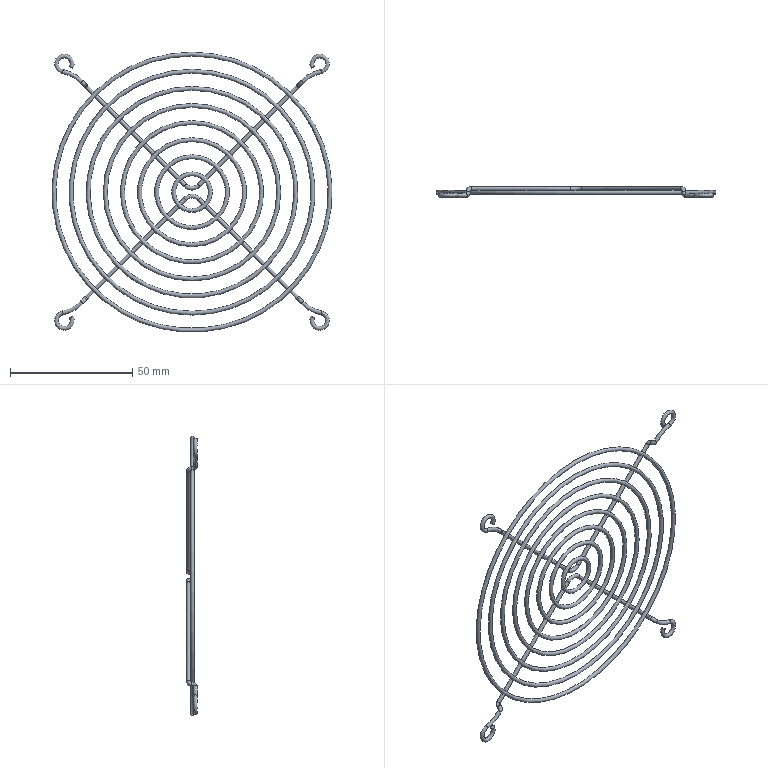Part | NX | features BREP 10 | 10 solids | 42 faces | box 114.6 x 4.4 x 114.6 mm | volume 3954 mm3 | torus 26 | plane 12 | cylinder 4 | commonest cylinder face diameters 1.6 x4
STEP:
#1=CARTESIAN_POINT('',(-52.712,-1.2,-50.143));
#2=VERTEX_POINT('',#1);
#3=CARTESIAN_POINT('',(-52.862,-1.2,-49.357));
#4=DIRECTION('',(-0.9823,0.,-0.1875));
#5=DIRECTION('',(0.1875,0.,-0.9823));
#6=AXIS2_PLACEMENT_3D('',#3,#4,#5);
#7=CIRCLE('',#6,0.8);
#8=EDGE_CURVE('',#2,#2,#7,.T.);
#9=ORIENTED_EDGE('',*,*,#8,.F.);
#10=EDGE_LOOP('',(#9));
#11=FACE_BOUND('',#10,.T.);
#12=CARTESIAN_POINT('',(-45.113,-0.4,-45.113));
#13=VERTEX_POINT('',#12);
#14=CARTESIAN_POINT('',(-44.532,-1.2,-45.663));
#15=VERTEX_POINT('',#14);
#16=CARTESIAN_POINT('',(-45.113,-0.4,-45.113));
#17=CARTESIAN_POINT('',(-44.809,-0.4,-45.401));
#18=CARTESIAN_POINT('',(-44.532,-0.7811,-45.663));
#19=CARTESIAN_POINT('',(-44.532,-1.2,-45.663));
#20=B_SPLINE_CURVE_WITH_KNOTS('',3,(#16,#17,#18,#19),.UNSPECIFIED.,.F.,.F.,(4,4),(0.,1.),.UNSPECIFIED.);
#21=EDGE_CURVE('',#13,#15,#20,.T.);
#22=ORIENTED_EDGE('',*,*,#21,.T.);
#23=CARTESIAN_POINT('',(-45.113,-2.,-45.113));
#24=VERTEX_POINT('',#23);
#25=CARTESIAN_POINT('',(-44.54,-1.2,-45.671));
#26=CARTESIAN_POINT('',(-44.539,-1.623,-45.671));
#27=CARTESIAN_POINT('',(-44.812,-2.,-45.405));
#28=CARTESIAN_POINT('',(-45.113,-2.,-45.113));
#29=B_SPLINE_CURVE_WITH_KNOTS('',3,(#25,#26,#27,#28),.UNSPECIFIED.,.F.,.F.,(4,4),(0.,0.001252),.UNSPECIFIED.);
#30=EDGE_CURVE('',#15,#24,#29,.T.);
#31=ORIENTED_EDGE('',*,*,#30,.T.);
#32=CARTESIAN_POINT('',(-45.113,-1.2,-45.113));
#33=DIRECTION('',(-0.687,0.,-0.7266));
#34=DIRECTION('',(0.7266,0.,-0.687));
#35=AXIS2_PLACEMENT_3D('',#32,#33,#34);
#36=CIRCLE('',#35,0.8);
#37=EDGE_CURVE('',#24,#13,#36,.T.);
#38=ORIENTED_EDGE('',*,*,#37,.T.);
#39=EDGE_LOOP('',(#22,#31,#38));
#40=FACE_BOUND('',#39,.T.);
#41=CARTESIAN_POINT('',(-55.558,-1.2,-35.238));
#42=DIRECTION('',(0.,1.,0.));
#43=DIRECTION('',(0.,0.,-1.));
#44=AXIS2_PLACEMENT_3D('',#41,#42,#43);
#45=TOROIDAL_SURFACE('',#44,14.374,0.8);
#46=ADVANCED_FACE('',(#11,#40),#45,.T.);
#47=CARTESIAN_POINT('',(-50.126,-1.2,-51.405));
#48=VERTEX_POINT('',#47);
#49=CARTESIAN_POINT('',(-49.414,-1.2,-51.04));
#50=DIRECTION('',(-0.4563,0.,0.8898));
#51=DIRECTION('',(-0.8898,0.,-0.4563));
#52=AXIS2_PLACEMENT_3D('',#49,#50,#51);
#53=CIRCLE('',#52,0.8);
#54=EDGE_CURVE('',#48,#48,#53,.T.);
#55=ORIENTED_EDGE('',*,*,#54,.F.);
#56=EDGE_LOOP('',(#55));
#57=FACE_BOUND('',#56,.T.);
#58=ORIENTED_EDGE('',*,*,#8,.T.);
#59=EDGE_LOOP('',(#58));
#60=FACE_BOUND('',#59,.T.);
#61=CARTESIAN_POINT('',(-52.262,-1.2,-52.5));
#62=DIRECTION('',(0.,-1.,0.));
#63=DIRECTION('',(0.,0.,1.));
#64=AXIS2_PLACEMENT_3D('',#61,#62,#63);
#65=TOROIDAL_SURFACE('',#64,3.2,0.8);
#66=ADVANCED_FACE('',(#57,#60),#65,.T.);
#67=CARTESIAN_POINT('',(-43.558,0.2,-44.689));
#68=VERTEX_POINT('',#67);
#69=CARTESIAN_POINT('',(-44.123,0.2,-44.123));
#70=DIRECTION('',(0.,-1.,0.));
#71=DIRECTION('',(0.7071,0.,-0.7071));
#72=AXIS2_PLACEMENT_3D('',#69,#70,#71);
#73=CIRCLE('',#72,0.8);
#74=EDGE_CURVE('',#68,#68,#73,.T.);
#75=ORIENTED_EDGE('',*,*,#74,.T.);
#76=EDGE_LOOP('',(#75));
#77=FACE_BOUND('',#76,.T.);
#78=CARTESIAN_POINT('',(-45.113,-1.2,-45.113));
#79=DIRECTION('',(-0.7071,0.,-0.7071));
#80=DIRECTION('',(0.7071,0.,-0.7071));
#81=AXIS2_PLACEMENT_3D('',#78,#79,#80);
#82=CIRCLE('',#81,0.8);
#83=EDGE_CURVE('',#24,#13,#82,.T.);
#84=ORIENTED_EDGE('',*,*,#83,.F.);
#85=ORIENTED_EDGE('',*,*,#30,.F.);
#86=ORIENTED_EDGE('',*,*,#21,.F.);
#87=EDGE_LOOP('',(#84,#85,#86));
#88=FACE_BOUND('',#87,.T.);
#89=CARTESIAN_POINT('',(-45.113,0.2,-45.113));
#90=DIRECTION('',(-0.7071,0.,0.7071));
#91=DIRECTION('',(-0.7071,0.,-0.7071));
#92=AXIS2_PLACEMENT_3D('',#89,#90,#91);
#93=TOROIDAL_SURFACE('',#92,1.4,0.8);
#94=ADVANCED_FACE('',(#77,#88),#93,.T.);
#95=CARTESIAN_POINT('',(-42.568,1.6,-43.699));
#96=VERTEX_POINT('',#95);
#97=CARTESIAN_POINT('',(-43.134,1.6,-43.134));
#98=DIRECTION('',(0.7071,0.,0.7071));
#99=DIRECTION('',(0.7071,0.,-0.7071));
#100=AXIS2_PLACEMENT_3D('',#97,#98,#99);
#101=CIRCLE('',#100,0.8);
#102=EDGE_CURVE('',#96,#96,#101,.T.);
#103=ORIENTED_EDGE('',*,*,#102,.F.);
#104=EDGE_LOOP('',(#103));
#105=FACE_BOUND('',#104,.T.);
#106=ORIENTED_EDGE('',*,*,#74,.F.);
#107=EDGE_LOOP('',(#106));
#108=FACE_BOUND('',#107,.T.);
#109=CARTESIAN_POINT('',(-43.134,0.2,-43.134));
#110=DIRECTION('',(0.7071,0.,-0.7071));
#111=DIRECTION('',(0.7071,0.,0.7071));
#112=AXIS2_PLACEMENT_3D('',#109,#110,#111);
#113=TOROIDAL_SURFACE('',#112,1.4,0.8);
#114=ADVANCED_FACE('',(#105,#108),#113,.T.);
#115=CARTESIAN_POINT('',(50.126,-1.2,-51.405));
#116=VERTEX_POINT('',#115);
#117=CARTESIAN_POINT('',(49.414,-1.2,-51.04));
#118=DIRECTION('',(0.4563,0.,0.8898));
#119=DIRECTION('',(0.8898,0.,-0.4563));
#120=AXIS2_PLACEMENT_3D('',#117,#118,#119);
#121=CIRCLE('',#120,0.8);
#122=EDGE_CURVE('',#116,#116,#121,.T.);
#123=ORIENTED_EDGE('',*,*,#122,.F.);
#124=EDGE_LOOP('',(#123));
#125=FACE_BOUND('',#124,.T.);
#126=CARTESIAN_POINT('',(52.712,-1.2,-50.143));
#127=VERTEX_POINT('',#126);
#128=CARTESIAN_POINT('',(52.862,-1.2,-49.357));
#129=DIRECTION('',(0.9823,0.,-0.1875));
#130=DIRECTION('',(-0.1875,0.,-0.9823));
#131=AXIS2_PLACEMENT_3D('',#128,#129,#130);
#132=CIRCLE('',#131,0.8);
#133=EDGE_CURVE('',#127,#127,#132,.T.);
#134=ORIENTED_EDGE('',*,*,#133,.T.);
#135=EDGE_LOOP('',(#134));
#136=FACE_BOUND('',#135,.T.);
#137=CARTESIAN_POINT('',(52.262,-1.2,-52.5));
#138=DIRECTION('',(0.,1.,0.));
#139=DIRECTION('',(0.,0.,-1.));
#140=AXIS2_PLACEMENT_3D('',#137,#138,#139);
#141=TOROIDAL_SURFACE('',#140,3.2,0.8);
#142=ADVANCED_FACE('',(#125,#136),#141,.T.);
#143=ORIENTED_EDGE('',*,*,#133,.F.);
#144=EDGE_LOOP('',(#143));
#145=FACE_BOUND('',#144,.T.);
#146=CARTESIAN_POINT('',(45.113,-2.,-45.113));
#147=VERTEX_POINT('',#146);
#148=CARTESIAN_POINT('',(44.538,-1.2,-45.67));
#149=VERTEX_POINT('',#148);
#150=CARTESIAN_POINT('',(45.113,-2.,-45.113));
#151=CARTESIAN_POINT('',(44.906,-2.,-45.321));
#152=CARTESIAN_POINT('',(44.583,-1.678,-45.641));
#153=CARTESIAN_POINT('',(44.542,-1.326,-45.674));
#154=CARTESIAN_POINT('',(44.539,-1.2,-45.67));
#155=B_SPLINE_CURVE_WITH_KNOTS('',3,(#150,#151,#152,#153,#154),.UNSPECIFIED.,.F.,.F.,(4,1,4),(0.,0.5,1.),.UNSPECIFIED.);
#156=EDGE_CURVE('',#147,#149,#155,.T.);
#157=ORIENTED_EDGE('',*,*,#156,.T.);
#158=CARTESIAN_POINT('',(45.113,-0.4,-45.113));
#159=VERTEX_POINT('',#158);
#160=CARTESIAN_POINT('',(44.54,-1.2,-45.671));
#161=CARTESIAN_POINT('',(44.54,-0.7768,-45.672));
#162=CARTESIAN_POINT('',(44.814,-0.4,-45.407));
#163=CARTESIAN_POINT('',(45.113,-0.4,-45.113));
#164=B_SPLINE_CURVE_WITH_KNOTS('',3,(#160,#161,#162,#163),.UNSPECIFIED.,.F.,.F.,(4,4),(0.000000002,0.001252),.UNSPECIFIED.);
#165=EDGE_CURVE('',#149,#159,#164,.T.);
#166=ORIENTED_EDGE('',*,*,#165,.T.);
#167=CARTESIAN_POINT('',(45.113,-1.2,-45.113));
#168=DIRECTION('',(0.687,0.,-0.7266));
#169=DIRECTION('',(0.7266,0.,0.687));
#170=AXIS2_PLACEMENT_3D('',#167,#168,#169);
#171=CIRCLE('',#170,0.8);
#172=EDGE_CURVE('',#159,#147,#171,.T.);
#173=ORIENTED_EDGE('',*,*,#172,.T.);
#174=EDGE_LOOP('',(#157,#166,#173));
#175=FACE_BOUND('',#174,.T.);
#176=CARTESIAN_POINT('',(55.558,-1.2,-35.238));
#177=DIRECTION('',(0.,-1.,0.));
#178=DIRECTION('',(0.,0.,1.));
#179=AXIS2_PLACEMENT_3D('',#176,#177,#178);
#180=TOROIDAL_SURFACE('',#179,14.374,0.8);
#181=ADVANCED_FACE('',(#145,#175),#180,.T.);
#182=CARTESIAN_POINT('',(43.558,0.2,-44.689));
#183=VERTEX_POINT('',#182);
#184=CARTESIAN_POINT('',(44.123,0.2,-44.123));
#185=DIRECTION('',(0.,-1.,0.));
#186=DIRECTION('',(-0.7071,0.,-0.7071));
#187=AXIS2_PLACEMENT_3D('',#184,#185,#186);
#188=CIRCLE('',#187,0.8);
#189=EDGE_CURVE('',#183,#183,#188,.T.);
#190=ORIENTED_EDGE('',*,*,#189,.T.);
#191=EDGE_LOOP('',(#190));
#192=FACE_BOUND('',#191,.T.);
#193=ORIENTED_EDGE('',*,*,#156,.F.);
#194=CARTESIAN_POINT('',(45.113,-1.2,-45.113));
#195=DIRECTION('',(0.7071,0.,-0.7071));
#196=DIRECTION('',(-0.7071,0.,-0.7071));
#197=AXIS2_PLACEMENT_3D('',#194,#195,#196);
#198=CIRCLE('',#197,0.8);
#199=EDGE_CURVE('',#159,#147,#198,.T.);
#200=ORIENTED_EDGE('',*,*,#199,.F.);
#201=ORIENTED_EDGE('',*,*,#165,.F.);
#202=EDGE_LOOP('',(#193,#200,#201));
#203=FACE_BOUND('',#202,.T.);
#204=CARTESIAN_POINT('',(45.113,0.2,-45.113));
#205=DIRECTION('',(-0.7071,0.,-0.7071));
#206=DIRECTION('',(0.7071,0.,-0.7071));
#207=AXIS2_PLACEMENT_3D('',#204,#205,#206);
#208=TOROIDAL_SURFACE('',#207,1.4,0.8);
#209=ADVANCED_FACE('',(#192,#203),#208,.T.);
#210=CARTESIAN_POINT('',(42.568,1.6,-43.699));
#211=VERTEX_POINT('',#210);
#212=CARTESIAN_POINT('',(43.134,1.6,-43.134));
#213=DIRECTION('',(0.7071,0.,-0.7071));
#214=DIRECTION('',(-0.7071,0.,-0.7071));
#215=AXIS2_PLACEMENT_3D('',#212,#213,#214);
#216=CIRCLE('',#215,0.8);
#217=EDGE_CURVE('',#211,#211,#216,.T.);
#218=ORIENTED_EDGE('',*,*,#217,.T.);
#219=EDGE_LOOP('',(#218));
#220=FACE_BOUND('',#219,.T.);
#221=ORIENTED_EDGE('',*,*,#189,.F.);
#222=EDGE_LOOP('',(#221));
#223=FACE_BOUND('',#222,.T.);
#224=CARTESIAN_POINT('',(43.134,0.2,-43.134));
#225=DIRECTION('',(0.7071,0.,0.7071));
#226=DIRECTION('',(-0.7071,0.,0.7071));
#227=AXIS2_PLACEMENT_3D('',#224,#225,#226);
#228=TOROIDAL_SURFACE('',#227,1.4,0.8);
#229=ADVANCED_FACE('',(#220,#223),#228,.T.);
#230=CARTESIAN_POINT('',(2.263,1.6,-3.394));
#231=VERTEX_POINT('',#230);
#232=CARTESIAN_POINT('',(2.828,1.6,-2.828));
#233=DIRECTION('',(0.7071,0.,-0.7071));
#234=DIRECTION('',(-0.7071,0.,-0.7071));
#235=AXIS2_PLACEMENT_3D('',#232,#233,#234);
#236=CIRCLE('',#235,0.8);
#237=EDGE_CURVE('',#231,#231,#236,.T.);
#238=ORIENTED_EDGE('',*,*,#237,.F.);
#239=EDGE_LOOP('',(#238));
#240=FACE_BOUND('',#239,.T.);
#241=CARTESIAN_POINT('',(-2.263,1.6,-3.394));
#242=VERTEX_POINT('',#241);
#243=CARTESIAN_POINT('',(-2.828,1.6,-2.828));
#244=DIRECTION('',(0.7071,0.,0.7071));
#245=DIRECTION('',(0.7071,0.,-0.7071));
#246=AXIS2_PLACEMENT_3D('',#243,#244,#245);
#247=CIRCLE('',#246,0.8);
#248=EDGE_CURVE('',#242,#242,#247,.T.);
#249=ORIENTED_EDGE('',*,*,#248,.T.);
#250=EDGE_LOOP('',(#249));
#251=FACE_BOUND('',#250,.T.);
#252=CARTESIAN_POINT('',(0.,1.6,-5.657));
#253=DIRECTION('',(0.,1.,0.));
#254=DIRECTION('',(0.,0.,-1.));
#255=AXIS2_PLACEMENT_3D('',#252,#253,#254);
#256=TOROIDAL_SURFACE('',#255,4.,0.8);
#257=ADVANCED_FACE('',(#240,#251),#256,.T.);
#258=ORIENTED_EDGE('',*,*,#102,.T.);
#259=EDGE_LOOP('',(#258));
#260=FACE_BOUND('',#259,.T.);
#261=ORIENTED_EDGE('',*,*,#248,.F.);
#262=EDGE_LOOP('',(#261));
#263=FACE_BOUND('',#262,.T.);
#264=CARTESIAN_POINT('',(-2.828,1.6,-2.828));
#265=DIRECTION('',(-0.7071,0.,-0.7071));
#266=DIRECTION('',(0.7071,0.,-0.7071));
#267=AXIS2_PLACEMENT_3D('',#264,#265,#266);
#268=CYLINDRICAL_SURFACE('',#267,0.8);
#269=ADVANCED_FACE('',(#260,#263),#268,.T.);
#270=ORIENTED_EDGE('',*,*,#237,.T.);
#271=EDGE_LOOP('',(#270));
#272=FACE_BOUND('',#271,.T.);
#273=ORIENTED_EDGE('',*,*,#217,.F.);
#274=EDGE_LOOP('',(#273));
#275=FACE_BOUND('',#274,.T.);
#276=CARTESIAN_POINT('',(43.134,1.6,-43.134));
#277=DIRECTION('',(-0.7071,0.,0.7071));
#278=DIRECTION('',(-0.7071,0.,-0.7071));
#279=AXIS2_PLACEMENT_3D('',#276,#277,#278);
#280=CYLINDRICAL_SURFACE('',#279,0.8);
#281=ADVANCED_FACE('',(#272,#275),#280,.T.);
#282=ORIENTED_EDGE('',*,*,#199,.T.);
#283=CARTESIAN_POINT('',(45.113,-1.2,-45.113));
#284=DIRECTION('',(0.,-1.,0.));
#285=VECTOR('',#284,1000.);
#286=LINE('',#283,#285);
#287=EDGE_CURVE('',#159,#147,#286,.T.);
#288=ORIENTED_EDGE('',*,*,#287,.F.);
#289=EDGE_LOOP('',(#282,#288));
#290=FACE_BOUND('',#289,.T.);
#291=CARTESIAN_POINT('',(45.113,-1.2,-45.113));
#292=DIRECTION('',(-0.7071,0.,0.7071));
#293=DIRECTION('',(-0.7071,0.,-0.7071));
#294=AXIS2_PLACEMENT_3D('',#291,#292,#293);
#295=PLANE('',#294);
#296=ADVANCED_FACE('',(#290),#295,.F.);
#297=ORIENTED_EDGE('',*,*,#287,.T.);
#298=ORIENTED_EDGE('',*,*,#172,.F.);
#299=EDGE_LOOP('',(#297,#298));
#300=FACE_BOUND('',#299,.T.);
#301=CARTESIAN_POINT('',(45.113,-1.2,-45.113));
#302=DIRECTION('',(-0.687,0.,0.7266));
#303=DIRECTION('',(-0.7266,0.,-0.687));
#304=AXIS2_PLACEMENT_3D('',#301,#302,#303);
#305=PLANE('',#304);
#306=ADVANCED_FACE('',(#300),#305,.T.);
#307=ORIENTED_EDGE('',*,*,#122,.T.);
#308=EDGE_LOOP('',(#307));
#309=FACE_BOUND('',#308,.T.);
#310=CARTESIAN_POINT('',(49.414,-1.2,-51.04));
#311=DIRECTION('',(-0.4563,0.,-0.8898));
#312=DIRECTION('',(0.8898,0.,-0.4563));
#313=AXIS2_PLACEMENT_3D('',#310,#311,#312);
#314=PLANE('',#313);
#315=ADVANCED_FACE('',(#309),#314,.F.);
#316=ORIENTED_EDGE('',*,*,#83,.T.);
#317=CARTESIAN_POINT('',(-45.113,-1.2,-45.113));
#318=DIRECTION('',(0.,1.,0.));
#319=VECTOR('',#318,1000.);
#320=LINE('',#317,#319);
#321=EDGE_CURVE('',#24,#13,#320,.T.);
#322=ORIENTED_EDGE('',*,*,#321,.F.);
#323=EDGE_LOOP('',(#316,#322));
#324=FACE_BOUND('',#323,.T.);
#325=CARTESIAN_POINT('',(-45.113,-1.2,-45.113));
#326=DIRECTION('',(0.7071,0.,0.7071));
#327=DIRECTION('',(0.7071,0.,-0.7071));
#328=AXIS2_PLACEMENT_3D('',#325,#326,#327);
#329=PLANE('',#328);
#330=ADVANCED_FACE('',(#324),#329,.F.);
#331=ORIENTED_EDGE('',*,*,#321,.T.);
#332=ORIENTED_EDGE('',*,*,#37,.F.);
#333=EDGE_LOOP('',(#331,#332));
#334=FACE_BOUND('',#333,.T.);
#335=CARTESIAN_POINT('',(-45.113,-1.2,-45.113));
#336=DIRECTION('',(0.687,0.,0.7266));
#337=DIRECTION('',(0.7266,0.,-0.687));
#338=AXIS2_PLACEMENT_3D('',#335,#336,#337);
#339=PLANE('',#338);
#340=ADVANCED_FACE('',(#334),#339,.T.);
#341=ORIENTED_EDGE('',*,*,#54,.T.);
#342=EDGE_LOOP('',(#341));
#343=FACE_BOUND('',#342,.T.);
#344=CARTESIAN_POINT('',(-49.414,-1.2,-51.04));
#345=DIRECTION('',(0.4563,0.,-0.8898));
#346=DIRECTION('',(-0.8898,0.,-0.4563));
#347=AXIS2_PLACEMENT_3D('',#344,#345,#346);
#348=PLANE('',#347);
#349=ADVANCED_FACE('',(#343),#348,.F.);
#350=CLOSED_SHELL('',(#46,#66,#94,#114,#142,#181,#209,#229,#257,#269,#281,#296,#306,#315,#330,#340,#349));
#351=MANIFOLD_SOLID_BREP('',#350);
#352=CARTESIAN_POINT('',(0.,0.,20.7));
#353=VERTEX_POINT('',#352);
#354=VERTEX_LOOP('',#353);
#355=FACE_BOUND('',#354,.T.);
#356=CARTESIAN_POINT('',(0.,0.,0.));
#357=DIRECTION('',(0.,1.,0.));
#358=DIRECTION('',(0.,0.,1.));
#359=AXIS2_PLACEMENT_3D('',#356,#357,#358);
#360=TOROIDAL_SURFACE('',#359,21.5,0.8);
#361=ADVANCED_FACE('',(#355),#360,.T.);
#362=CLOSED_SHELL('',(#361));
#363=MANIFOLD_SOLID_BREP('',#362);
#364=CARTESIAN_POINT('',(0.,0.,27.7));
#365=VERTEX_POINT('',#364);
#366=VERTEX_LOOP('',#365);
#367=FACE_BOUND('',#366,.T.);
#368=CARTESIAN_POINT('',(0.,0.,0.));
#369=DIRECTION('',(0.,1.,0.));
#370=DIRECTION('',(0.,0.,1.));
#371=AXIS2_PLACEMENT_3D('',#368,#369,#370);
#372=TOROIDAL_SURFACE('',#371,28.5,0.8);
#373=ADVANCED_FACE('',(#367),#372,.T.);
#374=CLOSED_SHELL('',(#373));
#375=MANIFOLD_SOLID_BREP('',#374);
#376=CARTESIAN_POINT('',(0.,0.,34.7));
#377=VERTEX_POINT('',#376);
#378=VERTEX_LOOP('',#377);
#379=FACE_BOUND('',#378,.T.);
#380=CARTESIAN_POINT('',(0.,0.,0.));
#381=DIRECTION('',(0.,1.,0.));
#382=DIRECTION('',(0.,0.,1.));
#383=AXIS2_PLACEMENT_3D('',#380,#381,#382);
#384=TOROIDAL_SURFACE('',#383,35.5,0.8);
#385=ADVANCED_FACE('',(#379),#384,.T.);
#386=CLOSED_SHELL('',(#385));
#387=MANIFOLD_SOLID_BREP('',#386);
#388=CARTESIAN_POINT('',(-45.113,-2.,45.113));
#389=VERTEX_POINT('',#388);
#390=CARTESIAN_POINT('',(-45.113,-0.4,45.113));
#391=VERTEX_POINT('',#390);
#392=CARTESIAN_POINT('',(-45.113,-1.2,45.113));
#393=DIRECTION('',(0.687,0.,-0.7266));
#394=DIRECTION('',(0.7266,0.,0.687));
#395=AXIS2_PLACEMENT_3D('',#392,#393,#394);
#396=CIRCLE('',#395,0.8);
#397=EDGE_CURVE('',#389,#391,#396,.T.);
#398=ORIENTED_EDGE('',*,*,#397,.F.);
#399=CARTESIAN_POINT('',(-44.532,-1.2,45.663));
#400=VERTEX_POINT('',#399);
#401=CARTESIAN_POINT('',(-44.54,-1.2,45.671));
#402=CARTESIAN_POINT('',(-44.539,-1.623,45.671));
#403=CARTESIAN_POINT('',(-44.812,-2.,45.405));
#404=CARTESIAN_POINT('',(-45.113,-2.,45.113));
#405=B_SPLINE_CURVE_WITH_KNOTS('',3,(#401,#402,#403,#404),.UNSPECIFIED.,.F.,.F.,(4,4),(0.,0.001252),.UNSPECIFIED.);
#406=EDGE_CURVE('',#400,#389,#405,.T.);
#407=ORIENTED_EDGE('',*,*,#406,.F.);
#408=CARTESIAN_POINT('',(-44.54,-1.2,45.671));
#409=CARTESIAN_POINT('',(-44.54,-0.7768,45.672));
#410=CARTESIAN_POINT('',(-44.814,-0.4,45.407));
#411=CARTESIAN_POINT('',(-45.113,-0.4,45.113));
#412=B_SPLINE_CURVE_WITH_KNOTS('',3,(#408,#409,#410,#411),.UNSPECIFIED.,.F.,.F.,(4,4),(0.000000067,0.001252),.UNSPECIFIED.);
#413=EDGE_CURVE('',#391,#400,#412,.F.);
#414=ORIENTED_EDGE('',*,*,#413,.F.);
#415=EDGE_LOOP('',(#398,#407,#414));
#416=FACE_BOUND('',#415,.T.);
#417=CARTESIAN_POINT('',(-52.712,-1.2,50.143));
#418=VERTEX_POINT('',#417);
#419=CARTESIAN_POINT('',(-52.862,-1.2,49.357));
#420=DIRECTION('',(0.9823,0.,-0.1875));
#421=DIRECTION('',(0.1875,0.,0.9823));
#422=AXIS2_PLACEMENT_3D('',#419,#420,#421);
#423=CIRCLE('',#422,0.8);
#424=EDGE_CURVE('',#418,#418,#423,.T.);
#425=ORIENTED_EDGE('',*,*,#424,.T.);
#426=EDGE_LOOP('',(#425));
#427=FACE_BOUND('',#426,.T.);
#428=CARTESIAN_POINT('',(-55.558,-1.2,35.238));
#429=DIRECTION('',(0.,1.,0.));
#430=DIRECTION('',(0.,0.,1.));
#431=AXIS2_PLACEMENT_3D('',#428,#429,#430);
#432=TOROIDAL_SURFACE('',#431,14.374,0.8);
#433=ADVANCED_FACE('',(#416,#427),#432,.T.);
#434=ORIENTED_EDGE('',*,*,#424,.F.);
#435=EDGE_LOOP('',(#434));
#436=FACE_BOUND('',#435,.T.);
#437=CARTESIAN_POINT('',(-50.126,-1.2,51.405));
#438=VERTEX_POINT('',#437);
#439=CARTESIAN_POINT('',(-49.414,-1.2,51.04));
#440=DIRECTION('',(0.4563,0.,0.8898));
#441=DIRECTION('',(-0.8898,0.,0.4563));
#442=AXIS2_PLACEMENT_3D('',#439,#440,#441);
#443=CIRCLE('',#442,0.8);
#444=EDGE_CURVE('',#438,#438,#443,.T.);
#445=ORIENTED_EDGE('',*,*,#444,.T.);
#446=EDGE_LOOP('',(#445));
#447=FACE_BOUND('',#446,.T.);
#448=CARTESIAN_POINT('',(-52.262,-1.2,52.5));
#449=DIRECTION('',(0.,-1.,0.));
#450=DIRECTION('',(0.,0.,-1.));
#451=AXIS2_PLACEMENT_3D('',#448,#449,#450);
#452=TOROIDAL_SURFACE('',#451,3.2,0.8);
#453=ADVANCED_FACE('',(#436,#447),#452,.T.);
#454=CARTESIAN_POINT('',(-45.113,-1.2,45.113));
#455=DIRECTION('',(0.7071,0.,-0.7071));
#456=DIRECTION('',(0.7071,0.,0.7071));
#457=AXIS2_PLACEMENT_3D('',#454,#455,#456);
#458=CIRCLE('',#457,0.8);
#459=EDGE_CURVE('',#389,#391,#458,.T.);
#460=ORIENTED_EDGE('',*,*,#459,.T.);
#461=ORIENTED_EDGE('',*,*,#413,.T.);
#462=ORIENTED_EDGE('',*,*,#406,.T.);
#463=EDGE_LOOP('',(#460,#461,#462));
#464=FACE_BOUND('',#463,.T.);
#465=CARTESIAN_POINT('',(-43.558,0.2,44.689));
#466=VERTEX_POINT('',#465);
#467=CARTESIAN_POINT('',(-44.123,0.2,44.123));
#468=DIRECTION('',(0.,1.,0.));
#469=DIRECTION('',(0.7071,0.,0.7071));
#470=AXIS2_PLACEMENT_3D('',#467,#468,#469);
#471=CIRCLE('',#470,0.8);
#472=EDGE_CURVE('',#466,#466,#471,.T.);
#473=ORIENTED_EDGE('',*,*,#472,.F.);
#474=EDGE_LOOP('',(#473));
#475=FACE_BOUND('',#474,.T.);
#476=CARTESIAN_POINT('',(-45.113,0.2,45.113));
#477=DIRECTION('',(-0.7071,0.,-0.7071));
#478=DIRECTION('',(-0.7071,0.,0.7071));
#479=AXIS2_PLACEMENT_3D('',#476,#477,#478);
#480=TOROIDAL_SURFACE('',#479,1.4,0.8);
#481=ADVANCED_FACE('',(#464,#475),#480,.T.);
#482=ORIENTED_EDGE('',*,*,#472,.T.);
#483=EDGE_LOOP('',(#482));
#484=FACE_BOUND('',#483,.T.);
#485=CARTESIAN_POINT('',(-42.568,1.6,43.699));
#486=VERTEX_POINT('',#485);
#487=CARTESIAN_POINT('',(-43.134,1.6,43.134));
#488=DIRECTION('',(-0.7071,0.,0.7071));
#489=DIRECTION('',(0.7071,0.,0.7071));
#490=AXIS2_PLACEMENT_3D('',#487,#488,#489);
#491=CIRCLE('',#490,0.8);
#492=EDGE_CURVE('',#486,#486,#491,.T.);
#493=ORIENTED_EDGE('',*,*,#492,.T.);
#494=EDGE_LOOP('',(#493));
#495=FACE_BOUND('',#494,.T.);
#496=CARTESIAN_POINT('',(-43.134,0.2,43.134));
#497=DIRECTION('',(0.7071,0.,0.7071));
#498=DIRECTION('',(0.7071,0.,-0.7071));
#499=AXIS2_PLACEMENT_3D('',#496,#497,#498);
#500=TOROIDAL_SURFACE('',#499,1.4,0.8);
#501=ADVANCED_FACE('',(#484,#495),#500,.T.);
#502=CARTESIAN_POINT('',(52.712,-1.2,50.143));
#503=VERTEX_POINT('',#502);
#504=CARTESIAN_POINT('',(52.862,-1.2,49.357));
#505=DIRECTION('',(-0.9823,0.,-0.1875));
#506=DIRECTION('',(-0.1875,0.,0.9823));
#507=AXIS2_PLACEMENT_3D('',#504,#505,#506);
#508=CIRCLE('',#507,0.8);
#509=EDGE_CURVE('',#503,#503,#508,.T.);
#510=ORIENTED_EDGE('',*,*,#509,.F.);
#511=EDGE_LOOP('',(#510));
#512=FACE_BOUND('',#511,.T.);
#513=CARTESIAN_POINT('',(50.126,-1.2,51.405));
#514=VERTEX_POINT('',#513);
#515=CARTESIAN_POINT('',(49.414,-1.2,51.04));
#516=DIRECTION('',(-0.4563,0.,0.8898));
#517=DIRECTION('',(0.8898,0.,0.4563));
#518=AXIS2_PLACEMENT_3D('',#515,#516,#517);
#519=CIRCLE('',#518,0.8);
#520=EDGE_CURVE('',#514,#514,#519,.T.);
#521=ORIENTED_EDGE('',*,*,#520,.T.);
#522=EDGE_LOOP('',(#521));
#523=FACE_BOUND('',#522,.T.);
#524=CARTESIAN_POINT('',(52.262,-1.2,52.5));
#525=DIRECTION('',(0.,1.,0.));
#526=DIRECTION('',(0.,0.,1.));
#527=AXIS2_PLACEMENT_3D('',#524,#525,#526);
#528=TOROIDAL_SURFACE('',#527,3.2,0.8);
#529=ADVANCED_FACE('',(#512,#523),#528,.T.);
#530=CARTESIAN_POINT('',(45.113,-0.4,45.113));
#531=VERTEX_POINT('',#530);
#532=CARTESIAN_POINT('',(45.113,-2.,45.113));
#533=VERTEX_POINT('',#532);
#534=CARTESIAN_POINT('',(45.113,-1.2,45.113));
#535=DIRECTION('',(-0.687,0.,-0.7266));
#536=DIRECTION('',(-0.7266,0.,0.687));
#537=AXIS2_PLACEMENT_3D('',#534,#535,#536);
#538=CIRCLE('',#537,0.8);
#539=EDGE_CURVE('',#531,#533,#538,.T.);
#540=ORIENTED_EDGE('',*,*,#539,.F.);
#541=CARTESIAN_POINT('',(44.54,-1.2,45.671));
#542=VERTEX_POINT('',#541);
#543=CARTESIAN_POINT('',(44.54,-1.2,45.671));
#544=CARTESIAN_POINT('',(44.54,-0.7768,45.672));
#545=CARTESIAN_POINT('',(44.814,-0.4,45.407));
#546=CARTESIAN_POINT('',(45.113,-0.4,45.113));
#547=B_SPLINE_CURVE_WITH_KNOTS('',3,(#543,#544,#545,#546),.UNSPECIFIED.,.F.,.F.,(4,4),(0.000000002,0.001252),.UNSPECIFIED.);
#548=EDGE_CURVE('',#542,#531,#547,.T.);
#549=ORIENTED_EDGE('',*,*,#548,.F.);
#550=CARTESIAN_POINT('',(44.54,-1.2,45.671));
#551=CARTESIAN_POINT('',(44.539,-1.623,45.671));
#552=CARTESIAN_POINT('',(44.812,-2.,45.405));
#553=CARTESIAN_POINT('',(45.113,-2.,45.113));
#554=B_SPLINE_CURVE_WITH_KNOTS('',3,(#550,#551,#552,#553),.UNSPECIFIED.,.F.,.F.,(4,4),(0.,0.001252),.UNSPECIFIED.);
#555=EDGE_CURVE('',#533,#542,#554,.F.);
#556=ORIENTED_EDGE('',*,*,#555,.F.);
#557=EDGE_LOOP('',(#540,#549,#556));
#558=FACE_BOUND('',#557,.T.);
#559=ORIENTED_EDGE('',*,*,#509,.T.);
#560=EDGE_LOOP('',(#559));
#561=FACE_BOUND('',#560,.T.);
#562=CARTESIAN_POINT('',(55.558,-1.2,35.238));
#563=DIRECTION('',(0.,-1.,0.));
#564=DIRECTION('',(0.,0.,-1.));
#565=AXIS2_PLACEMENT_3D('',#562,#563,#564);
#566=TOROIDAL_SURFACE('',#565,14.374,0.8);
#567=ADVANCED_FACE('',(#558,#561),#566,.T.);
#568=ORIENTED_EDGE('',*,*,#548,.T.);
#569=CARTESIAN_POINT('',(45.113,-1.2,45.113));
#570=DIRECTION('',(-0.7071,0.,-0.7071));
#571=DIRECTION('',(-0.7071,0.,0.7071));
#572=AXIS2_PLACEMENT_3D('',#569,#570,#571);
#573=CIRCLE('',#572,0.8);
#574=EDGE_CURVE('',#531,#533,#573,.T.);
#575=ORIENTED_EDGE('',*,*,#574,.T.);
#576=ORIENTED_EDGE('',*,*,#555,.T.);
#577=EDGE_LOOP('',(#568,#575,#576));
#578=FACE_BOUND('',#577,.T.);
#579=CARTESIAN_POINT('',(43.558,0.2,44.689));
#580=VERTEX_POINT('',#579);
#581=CARTESIAN_POINT('',(44.123,0.2,44.123));
#582=DIRECTION('',(0.,1.,0.));
#583=DIRECTION('',(-0.7071,0.,0.7071));
#584=AXIS2_PLACEMENT_3D('',#581,#582,#583);
#585=CIRCLE('',#584,0.8);
#586=EDGE_CURVE('',#580,#580,#585,.T.);
#587=ORIENTED_EDGE('',*,*,#586,.F.);
#588=EDGE_LOOP('',(#587));
#589=FACE_BOUND('',#588,.T.);
#590=CARTESIAN_POINT('',(45.113,0.2,45.113));
#591=DIRECTION('',(-0.7071,0.,0.7071));
#592=DIRECTION('',(0.7071,0.,0.7071));
#593=AXIS2_PLACEMENT_3D('',#590,#591,#592);
#594=TOROIDAL_SURFACE('',#593,1.4,0.8);
#595=ADVANCED_FACE('',(#578,#589),#594,.T.);
#596=ORIENTED_EDGE('',*,*,#586,.T.);
#597=EDGE_LOOP('',(#596));
#598=FACE_BOUND('',#597,.T.);
#599=CARTESIAN_POINT('',(42.568,1.6,43.699));
#600=VERTEX_POINT('',#599);
#601=CARTESIAN_POINT('',(43.134,1.6,43.134));
#602=DIRECTION('',(-0.7071,0.,-0.7071));
#603=DIRECTION('',(-0.7071,0.,0.7071));
#604=AXIS2_PLACEMENT_3D('',#601,#602,#603);
#605=CIRCLE('',#604,0.8);
#606=EDGE_CURVE('',#600,#600,#605,.T.);
#607=ORIENTED_EDGE('',*,*,#606,.F.);
#608=EDGE_LOOP('',(#607));
#609=FACE_BOUND('',#608,.T.);
#610=CARTESIAN_POINT('',(43.134,0.2,43.134));
#611=DIRECTION('',(0.7071,0.,-0.7071));
#612=DIRECTION('',(-0.7071,0.,-0.7071));
#613=AXIS2_PLACEMENT_3D('',#610,#611,#612);
#614=TOROIDAL_SURFACE('',#613,1.4,0.8);
#615=ADVANCED_FACE('',(#598,#609),#614,.T.);
#616=CARTESIAN_POINT('',(-2.263,1.6,3.394));
#617=VERTEX_POINT('',#616);
#618=CARTESIAN_POINT('',(-2.828,1.6,2.828));
#619=DIRECTION('',(-0.7071,0.,0.7071));
#620=DIRECTION('',(0.7071,0.,0.7071));
#621=AXIS2_PLACEMENT_3D('',#618,#619,#620);
#622=CIRCLE('',#621,0.8);
#623=EDGE_CURVE('',#617,#617,#622,.T.);
#624=ORIENTED_EDGE('',*,*,#623,.F.);
#625=EDGE_LOOP('',(#624));
#626=FACE_BOUND('',#625,.T.);
#627=CARTESIAN_POINT('',(2.263,1.6,3.394));
#628=VERTEX_POINT('',#627);
#629=CARTESIAN_POINT('',(2.828,1.6,2.828));
#630=DIRECTION('',(-0.7071,0.,-0.7071));
#631=DIRECTION('',(-0.7071,0.,0.7071));
#632=AXIS2_PLACEMENT_3D('',#629,#630,#631);
#633=CIRCLE('',#632,0.8);
#634=EDGE_CURVE('',#628,#628,#633,.T.);
#635=ORIENTED_EDGE('',*,*,#634,.T.);
#636=EDGE_LOOP('',(#635));
#637=FACE_BOUND('',#636,.T.);
#638=CARTESIAN_POINT('',(0.,1.6,5.657));
#639=DIRECTION('',(0.,1.,0.));
#640=DIRECTION('',(0.,0.,1.));
#641=AXIS2_PLACEMENT_3D('',#638,#639,#640);
#642=TOROIDAL_SURFACE('',#641,4.,0.8);
#643=ADVANCED_FACE('',(#626,#637),#642,.T.);
#644=ORIENTED_EDGE('',*,*,#492,.F.);
#645=EDGE_LOOP('',(#644));
#646=FACE_BOUND('',#645,.T.);
#647=ORIENTED_EDGE('',*,*,#623,.T.);
#648=EDGE_LOOP('',(#647));
#649=FACE_BOUND('',#648,.T.);
#650=CARTESIAN_POINT('',(-2.828,1.6,2.828));
#651=DIRECTION('',(-0.7071,0.,0.7071));
#652=DIRECTION('',(0.7071,0.,0.7071));
#653=AXIS2_PLACEMENT_3D('',#650,#651,#652);
#654=CYLINDRICAL_SURFACE('',#653,0.8);
#655=ADVANCED_FACE('',(#646,#649),#654,.T.);
#656=ORIENTED_EDGE('',*,*,#634,.F.);
#657=EDGE_LOOP('',(#656));
#658=FACE_BOUND('',#657,.T.);
#659=ORIENTED_EDGE('',*,*,#606,.T.);
#660=EDGE_LOOP('',(#659));
#661=FACE_BOUND('',#660,.T.);
#662=CARTESIAN_POINT('',(43.134,1.6,43.134));
#663=DIRECTION('',(-0.7071,0.,-0.7071));
#664=DIRECTION('',(-0.7071,0.,0.7071));
#665=AXIS2_PLACEMENT_3D('',#662,#663,#664);
#666=CYLINDRICAL_SURFACE('',#665,0.8);
#667=ADVANCED_FACE('',(#658,#661),#666,.T.);
#668=ORIENTED_EDGE('',*,*,#574,.F.);
#669=CARTESIAN_POINT('',(45.113,-1.2,45.113));
#670=DIRECTION('',(0.,-1.,0.));
#671=VECTOR('',#670,1000.);
#672=LINE('',#669,#671);
#673=EDGE_CURVE('',#531,#533,#672,.T.);
#674=ORIENTED_EDGE('',*,*,#673,.T.);
#675=EDGE_LOOP('',(#668,#674));
#676=FACE_BOUND('',#675,.T.);
#677=CARTESIAN_POINT('',(45.113,-1.2,45.113));
#678=DIRECTION('',(-0.7071,0.,-0.7071));
#679=DIRECTION('',(-0.7071,0.,0.7071));
#680=AXIS2_PLACEMENT_3D('',#677,#678,#679);
#681=PLANE('',#680);
#682=ADVANCED_FACE('',(#676),#681,.F.);
#683=ORIENTED_EDGE('',*,*,#673,.F.);
#684=ORIENTED_EDGE('',*,*,#539,.T.);
#685=EDGE_LOOP('',(#683,#684));
#686=FACE_BOUND('',#685,.T.);
#687=CARTESIAN_POINT('',(45.113,-1.2,45.113));
#688=DIRECTION('',(-0.687,0.,-0.7266));
#689=DIRECTION('',(-0.7266,0.,0.687));
#690=AXIS2_PLACEMENT_3D('',#687,#688,#689);
#691=PLANE('',#690);
#692=ADVANCED_FACE('',(#686),#691,.T.);
#693=ORIENTED_EDGE('',*,*,#520,.F.);
#694=EDGE_LOOP('',(#693));
#695=FACE_BOUND('',#694,.T.);
#696=CARTESIAN_POINT('',(49.414,-1.2,51.04));
#697=DIRECTION('',(-0.4563,0.,0.8898));
#698=DIRECTION('',(0.8898,0.,0.4563));
#699=AXIS2_PLACEMENT_3D('',#696,#697,#698);
#700=PLANE('',#699);
#701=ADVANCED_FACE('',(#695),#700,.F.);
#702=ORIENTED_EDGE('',*,*,#459,.F.);
#703=CARTESIAN_POINT('',(-45.113,-1.2,45.113));
#704=DIRECTION('',(0.,1.,0.));
#705=VECTOR('',#704,1000.);
#706=LINE('',#703,#705);
#707=EDGE_CURVE('',#389,#391,#706,.T.);
#708=ORIENTED_EDGE('',*,*,#707,.T.);
#709=EDGE_LOOP('',(#702,#708));
#710=FACE_BOUND('',#709,.T.);
#711=CARTESIAN_POINT('',(-45.113,-1.2,45.113));
#712=DIRECTION('',(0.7071,0.,-0.7071));
#713=DIRECTION('',(0.7071,0.,0.7071));
#714=AXIS2_PLACEMENT_3D('',#711,#712,#713);
#715=PLANE('',#714);
#716=ADVANCED_FACE('',(#710),#715,.F.);
#717=ORIENTED_EDGE('',*,*,#707,.F.);
#718=ORIENTED_EDGE('',*,*,#397,.T.);
#719=EDGE_LOOP('',(#717,#718));
#720=FACE_BOUND('',#719,.T.);
#721=CARTESIAN_POINT('',(-45.113,-1.2,45.113));
#722=DIRECTION('',(0.687,0.,-0.7266));
#723=DIRECTION('',(0.7266,0.,0.687));
#724=AXIS2_PLACEMENT_3D('',#721,#722,#723);
#725=PLANE('',#724);
#726=ADVANCED_FACE('',(#720),#725,.T.);
#727=ORIENTED_EDGE('',*,*,#444,.F.);
#728=EDGE_LOOP('',(#727));
#729=FACE_BOUND('',#728,.T.);
#730=CARTESIAN_POINT('',(-49.414,-1.2,51.04));
#731=DIRECTION('',(0.4563,0.,0.8898));
#732=DIRECTION('',(-0.8898,0.,0.4563));
#733=AXIS2_PLACEMENT_3D('',#730,#731,#732);
#734=PLANE('',#733);
#735=ADVANCED_FACE('',(#729),#734,.F.);
#736=CLOSED_SHELL('',(#433,#453,#481,#501,#529,#567,#595,#615,#643,#655,#667,#682,#692,#701,#716,#726,#735));
#737=MANIFOLD_SOLID_BREP('',#736);
#738=CARTESIAN_POINT('',(0.,0.,55.7));
#739=VERTEX_POINT('',#738);
#740=VERTEX_LOOP('',#739);
#741=FACE_BOUND('',#740,.T.);
#742=CARTESIAN_POINT('',(0.,0.,0.));
#743=DIRECTION('',(0.,1.,0.));
#744=DIRECTION('',(0.,0.,1.));
#745=AXIS2_PLACEMENT_3D('',#742,#743,#744);
#746=TOROIDAL_SURFACE('',#745,56.5,0.8);
#747=ADVANCED_FACE('',(#741),#746,.T.);
#748=CLOSED_SHELL('',(#747));
#749=MANIFOLD_SOLID_BREP('',#748);
#750=CARTESIAN_POINT('',(0.,0.,13.7));
#751=VERTEX_POINT('',#750);
#752=VERTEX_LOOP('',#751);
#753=FACE_BOUND('',#752,.T.);
#754=CARTESIAN_POINT('',(0.,0.,0.));
#755=DIRECTION('',(0.,1.,0.));
#756=DIRECTION('',(0.,0.,1.));
#757=AXIS2_PLACEMENT_3D('',#754,#755,#756);
#758=TOROIDAL_SURFACE('',#757,14.5,0.8);
#759=ADVANCED_FACE('',(#753),#758,.T.);
#760=CLOSED_SHELL('',(#759));
#761=MANIFOLD_SOLID_BREP('',#760);
#762=CARTESIAN_POINT('',(0.,0.,6.7));
#763=VERTEX_POINT('',#762);
#764=VERTEX_LOOP('',#763);
#765=FACE_BOUND('',#764,.T.);
#766=CARTESIAN_POINT('',(0.,0.,0.));
#767=DIRECTION('',(0.,1.,0.));
#768=DIRECTION('',(0.,0.,1.));
#769=AXIS2_PLACEMENT_3D('',#766,#767,#768);
#770=TOROIDAL_SURFACE('',#769,7.5,0.8);
#771=ADVANCED_FACE('',(#765),#770,.T.);
#772=CLOSED_SHELL('',(#771));
#773=MANIFOLD_SOLID_BREP('',#772);
#774=CARTESIAN_POINT('',(0.,0.,41.7));
#775=VERTEX_POINT('',#774);
#776=VERTEX_LOOP('',#775);
#777=FACE_BOUND('',#776,.T.);
#778=CARTESIAN_POINT('',(0.,0.,0.));
#779=DIRECTION('',(0.,1.,0.));
#780=DIRECTION('',(0.,0.,1.));
#781=AXIS2_PLACEMENT_3D('',#778,#779,#780);
#782=TOROIDAL_SURFACE('',#781,42.5,0.8);
#783=ADVANCED_FACE('',(#777),#782,.T.);
#784=CLOSED_SHELL('',(#783));
#785=MANIFOLD_SOLID_BREP('',#784);
#786=CARTESIAN_POINT('',(0.,0.,48.7));
#787=VERTEX_POINT('',#786);
#788=VERTEX_LOOP('',#787);
#789=FACE_BOUND('',#788,.T.);
#790=CARTESIAN_POINT('',(0.,0.,0.));
#791=DIRECTION('',(0.,1.,0.));
#792=DIRECTION('',(0.,0.,1.));
#793=AXIS2_PLACEMENT_3D('',#790,#791,#792);
#794=TOROIDAL_SURFACE('',#793,49.5,0.8);
#795=ADVANCED_FACE('',(#789),#794,.T.);
#796=CLOSED_SHELL('',(#795));
#797=MANIFOLD_SOLID_BREP('',#796);
#798=(LENGTH_UNIT()NAMED_UNIT(*)SI_UNIT(.MILLI.,.METRE.));
#799=UNCERTAINTY_MEASURE_WITH_UNIT(LENGTH_MEASURE(0.0508),#798,'','');
#800=(NAMED_UNIT(*)PLANE_ANGLE_UNIT()SI_UNIT($,.RADIAN.));
#801=(NAMED_UNIT(*)SI_UNIT($,.STERADIAN.)SOLID_ANGLE_UNIT());
#802=(GEOMETRIC_REPRESENTATION_CONTEXT(3)GLOBAL_UNCERTAINTY_ASSIGNED_CONTEXT((#799))GLOBAL_UNIT_ASSIGNED_CONTEXT((#798,#800,#801))REPRESENTATION_CONTEXT('',''));
#803=ADVANCED_BREP_SHAPE_REPRESENTATION('',(#351,#363,#375,#387,#737,#749,#761,#773,#785,#797),#802);